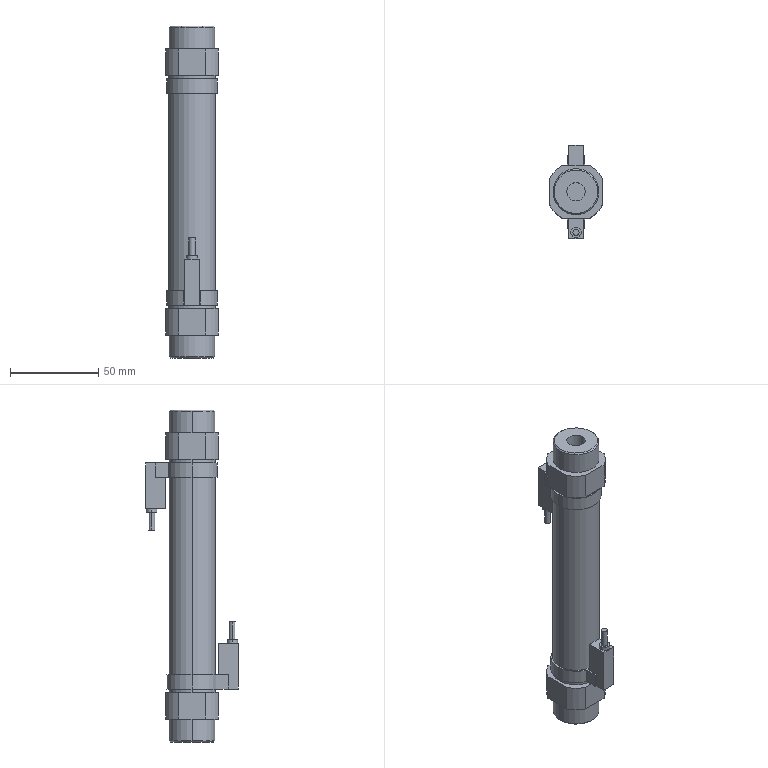Part | STEP file | body_A_CDM2B25_100_C76_0_ | 1 solid | 97 faces | box 30 x 52.6 x 188 mm | volume 108321 mm3 | plane 49 | cylinder 40 | cone 8 | commonest cylinder face diameters 28.6 x8 33.5 x8 26.6 x6 3.4 x4 6 x4 8.57 x4